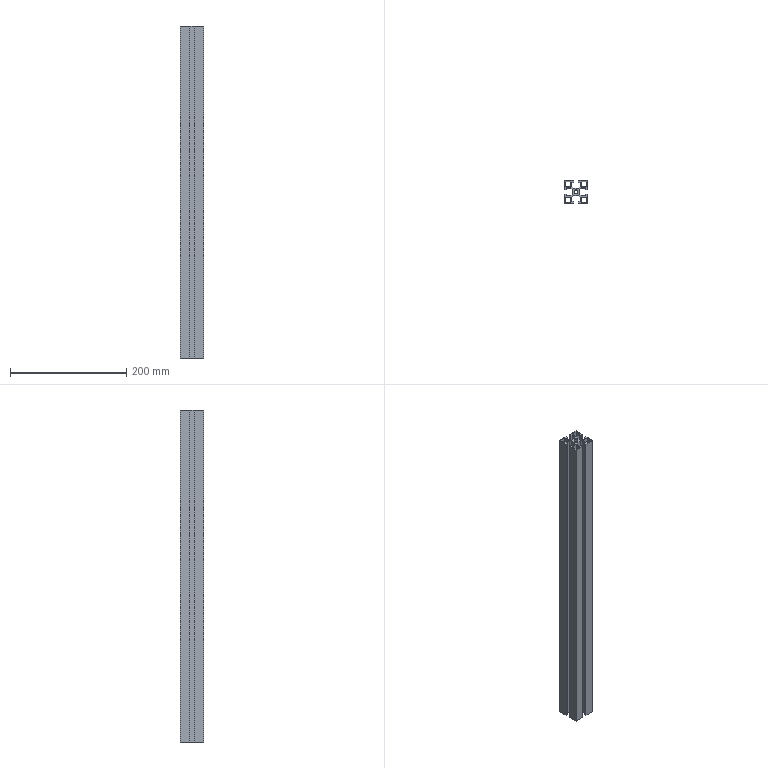Part | STEP file | 40-570-2 | 1 solid | 64 faces | box 40 x 40 x 570 mm | volume 299104 mm3 | plane 62 | cylinder 2 | commonest cylinder face diameters 6.8 x2